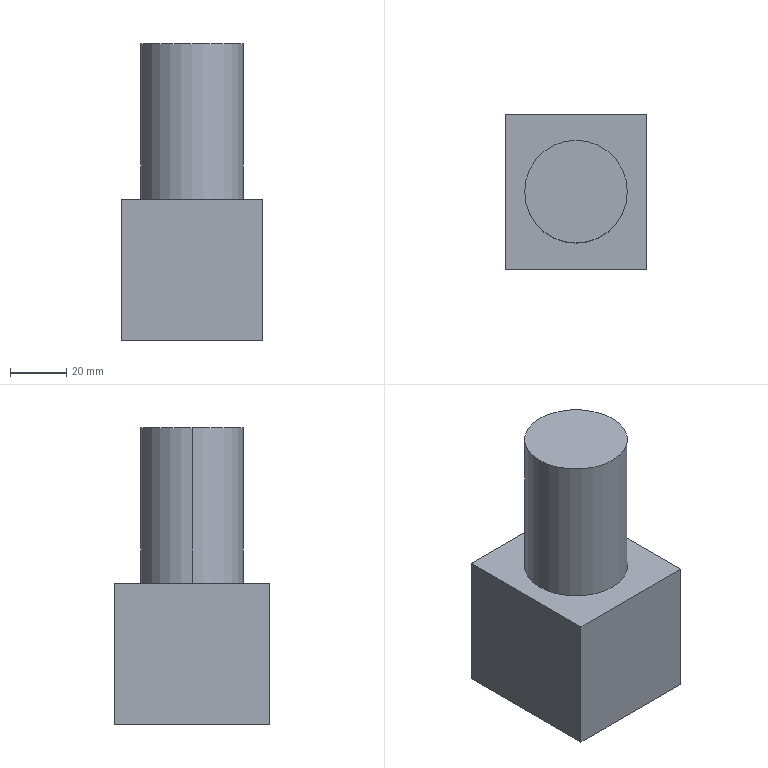Part | SolidWorks | features Extrusion 1, ICE 1 | 1 solid | 9 faces | box 50 x 55 x 105 mm | volume 194665 mm3 | plane 7 | cylinder 2 | commonest cylinder face diameters 36.378 x2
STEP:
#1=CARTESIAN_POINT('',(18.189,27.5,80.));
#2=VERTEX_POINT('',#1);
#3=CARTESIAN_POINT('',(-18.189,27.5,80.));
#4=VERTEX_POINT('',#3);
#5=CARTESIAN_POINT('',(0.,27.5,80.));
#6=DIRECTION('',(0.,0.,1.));
#7=DIRECTION('',(1.,0.,0.));
#8=AXIS2_PLACEMENT_3D('',#5,#6,#7);
#9=CIRCLE('',#8,18.189);
#10=EDGE_CURVE('',#2,#4,#9,.T.);
#11=ORIENTED_EDGE('',*,*,#10,.F.);
#12=CARTESIAN_POINT('',(18.189,27.5,25.));
#13=VERTEX_POINT('',#12);
#14=CARTESIAN_POINT('',(18.189,27.5,80.));
#15=DIRECTION('',(0.,0.,-1.));
#16=VECTOR('',#15,1000.);
#17=LINE('',#14,#16);
#18=EDGE_CURVE('',#2,#13,#17,.T.);
#19=ORIENTED_EDGE('',*,*,#18,.T.);
#20=CARTESIAN_POINT('',(-18.189,27.5,25.));
#21=VERTEX_POINT('',#20);
#22=CARTESIAN_POINT('',(0.,27.5,25.));
#23=DIRECTION('',(0.,0.,1.));
#24=DIRECTION('',(1.,0.,0.));
#25=AXIS2_PLACEMENT_3D('',#22,#23,#24);
#26=CIRCLE('',#25,18.189);
#27=EDGE_CURVE('',#13,#21,#26,.T.);
#28=ORIENTED_EDGE('',*,*,#27,.T.);
#29=CARTESIAN_POINT('',(-18.189,27.5,80.));
#30=DIRECTION('',(0.,0.,-1.));
#31=VECTOR('',#30,1000.);
#32=LINE('',#29,#31);
#33=EDGE_CURVE('',#4,#21,#32,.T.);
#34=ORIENTED_EDGE('',*,*,#33,.F.);
#35=EDGE_LOOP('',(#11,#19,#28,#34));
#36=FACE_OUTER_BOUND('',#35,.T.);
#37=CARTESIAN_POINT('',(0.,27.5,80.));
#38=DIRECTION('',(0.,0.,-1.));
#39=DIRECTION('',(-1.,0.,0.));
#40=AXIS2_PLACEMENT_3D('',#37,#38,#39);
#41=CYLINDRICAL_SURFACE('',#40,18.189);
#42=ADVANCED_FACE('',(#36),#41,.T.);
#43=CARTESIAN_POINT('',(25.,0.,25.));
#44=VERTEX_POINT('',#43);
#45=CARTESIAN_POINT('',(25.,0.,-25.));
#46=VERTEX_POINT('',#45);
#47=CARTESIAN_POINT('',(25.,0.,-25.));
#48=DIRECTION('',(0.,0.,-1.));
#49=VECTOR('',#48,1000.);
#50=LINE('',#47,#49);
#51=EDGE_CURVE('',#44,#46,#50,.T.);
#52=ORIENTED_EDGE('',*,*,#51,.T.);
#53=CARTESIAN_POINT('',(25.,55.,-25.));
#54=VERTEX_POINT('',#53);
#55=CARTESIAN_POINT('',(25.,55.,-25.));
#56=DIRECTION('',(0.,-1.,0.));
#57=VECTOR('',#56,1000.);
#58=LINE('',#55,#57);
#59=EDGE_CURVE('',#54,#46,#58,.T.);
#60=ORIENTED_EDGE('',*,*,#59,.F.);
#61=CARTESIAN_POINT('',(25.,55.,25.));
#62=VERTEX_POINT('',#61);
#63=CARTESIAN_POINT('',(25.,55.,-25.));
#64=DIRECTION('',(0.,0.,-1.));
#65=VECTOR('',#64,1000.);
#66=LINE('',#63,#65);
#67=EDGE_CURVE('',#62,#54,#66,.T.);
#68=ORIENTED_EDGE('',*,*,#67,.F.);
#69=CARTESIAN_POINT('',(25.,55.,25.));
#70=DIRECTION('',(0.,-1.,0.));
#71=VECTOR('',#70,1000.);
#72=LINE('',#69,#71);
#73=EDGE_CURVE('',#62,#44,#72,.T.);
#74=ORIENTED_EDGE('',*,*,#73,.T.);
#75=EDGE_LOOP('',(#52,#60,#68,#74));
#76=FACE_OUTER_BOUND('',#75,.T.);
#77=CARTESIAN_POINT('',(25.,55.,-25.));
#78=DIRECTION('',(-1.,0.,0.));
#79=DIRECTION('',(0.,0.,1.));
#80=AXIS2_PLACEMENT_3D('',#77,#78,#79);
#81=PLANE('',#80);
#82=ADVANCED_FACE('',(#76),#81,.F.);
#83=CARTESIAN_POINT('',(-25.,0.,-25.));
#84=VERTEX_POINT('',#83);
#85=CARTESIAN_POINT('',(-25.,0.,-25.));
#86=DIRECTION('',(-1.,0.,0.));
#87=VECTOR('',#86,1000.);
#88=LINE('',#85,#87);
#89=EDGE_CURVE('',#46,#84,#88,.T.);
#90=ORIENTED_EDGE('',*,*,#89,.T.);
#91=CARTESIAN_POINT('',(-25.,55.,-25.));
#92=VERTEX_POINT('',#91);
#93=CARTESIAN_POINT('',(-25.,55.,-25.));
#94=DIRECTION('',(0.,-1.,0.));
#95=VECTOR('',#94,1000.);
#96=LINE('',#93,#95);
#97=EDGE_CURVE('',#92,#84,#96,.T.);
#98=ORIENTED_EDGE('',*,*,#97,.F.);
#99=CARTESIAN_POINT('',(-25.,55.,-25.));
#100=DIRECTION('',(-1.,0.,0.));
#101=VECTOR('',#100,1000.);
#102=LINE('',#99,#101);
#103=EDGE_CURVE('',#54,#92,#102,.T.);
#104=ORIENTED_EDGE('',*,*,#103,.F.);
#105=ORIENTED_EDGE('',*,*,#59,.T.);
#106=EDGE_LOOP('',(#90,#98,#104,#105));
#107=FACE_OUTER_BOUND('',#106,.T.);
#108=CARTESIAN_POINT('',(-25.,55.,-25.));
#109=DIRECTION('',(0.,0.,1.));
#110=DIRECTION('',(1.,0.,0.));
#111=AXIS2_PLACEMENT_3D('',#108,#109,#110);
#112=PLANE('',#111);
#113=ADVANCED_FACE('',(#107),#112,.F.);
#114=CARTESIAN_POINT('',(-25.,0.,25.));
#115=VERTEX_POINT('',#114);
#116=CARTESIAN_POINT('',(-25.,0.,-25.));
#117=DIRECTION('',(0.,0.,1.));
#118=VECTOR('',#117,1000.);
#119=LINE('',#116,#118);
#120=EDGE_CURVE('',#84,#115,#119,.T.);
#121=ORIENTED_EDGE('',*,*,#120,.T.);
#122=CARTESIAN_POINT('',(-25.,55.,25.));
#123=VERTEX_POINT('',#122);
#124=CARTESIAN_POINT('',(-25.,55.,25.));
#125=DIRECTION('',(0.,-1.,0.));
#126=VECTOR('',#125,1000.);
#127=LINE('',#124,#126);
#128=EDGE_CURVE('',#123,#115,#127,.T.);
#129=ORIENTED_EDGE('',*,*,#128,.F.);
#130=CARTESIAN_POINT('',(-25.,55.,-25.));
#131=DIRECTION('',(0.,0.,1.));
#132=VECTOR('',#131,1000.);
#133=LINE('',#130,#132);
#134=EDGE_CURVE('',#92,#123,#133,.T.);
#135=ORIENTED_EDGE('',*,*,#134,.F.);
#136=ORIENTED_EDGE('',*,*,#97,.T.);
#137=EDGE_LOOP('',(#121,#129,#135,#136));
#138=FACE_OUTER_BOUND('',#137,.T.);
#139=CARTESIAN_POINT('',(-25.,55.,-25.));
#140=DIRECTION('',(1.,0.,0.));
#141=DIRECTION('',(0.,0.,-1.));
#142=AXIS2_PLACEMENT_3D('',#139,#140,#141);
#143=PLANE('',#142);
#144=ADVANCED_FACE('',(#138),#143,.F.);
#145=CARTESIAN_POINT('',(0.,27.5,25.));
#146=DIRECTION('',(0.,0.,1.));
#147=DIRECTION('',(1.,0.,0.));
#148=AXIS2_PLACEMENT_3D('',#145,#146,#147);
#149=CIRCLE('',#148,18.189);
#150=EDGE_CURVE('',#21,#13,#149,.T.);
#151=ORIENTED_EDGE('',*,*,#150,.F.);
#152=ORIENTED_EDGE('',*,*,#27,.F.);
#153=EDGE_LOOP('',(#151,#152));
#154=FACE_BOUND('',#153,.T.);
#155=CARTESIAN_POINT('',(-25.,0.,25.));
#156=DIRECTION('',(1.,0.,0.));
#157=VECTOR('',#156,1000.);
#158=LINE('',#155,#157);
#159=EDGE_CURVE('',#115,#44,#158,.T.);
#160=ORIENTED_EDGE('',*,*,#159,.T.);
#161=ORIENTED_EDGE('',*,*,#73,.F.);
#162=CARTESIAN_POINT('',(-25.,55.,25.));
#163=DIRECTION('',(1.,0.,0.));
#164=VECTOR('',#163,1000.);
#165=LINE('',#162,#164);
#166=EDGE_CURVE('',#123,#62,#165,.T.);
#167=ORIENTED_EDGE('',*,*,#166,.F.);
#168=ORIENTED_EDGE('',*,*,#128,.T.);
#169=EDGE_LOOP('',(#160,#161,#167,#168));
#170=FACE_OUTER_BOUND('',#169,.T.);
#171=CARTESIAN_POINT('',(-25.,55.,25.));
#172=DIRECTION('',(0.,0.,-1.));
#173=DIRECTION('',(-1.,0.,0.));
#174=AXIS2_PLACEMENT_3D('',#171,#172,#173);
#175=PLANE('',#174);
#176=ADVANCED_FACE('',(#154,#170),#175,.F.);
#177=ORIENTED_EDGE('',*,*,#67,.T.);
#178=ORIENTED_EDGE('',*,*,#103,.T.);
#179=ORIENTED_EDGE('',*,*,#134,.T.);
#180=ORIENTED_EDGE('',*,*,#166,.T.);
#181=EDGE_LOOP('',(#177,#178,#179,#180));
#182=FACE_OUTER_BOUND('',#181,.T.);
#183=CARTESIAN_POINT('',(0.,55.,0.));
#184=DIRECTION('',(0.,1.,0.));
#185=DIRECTION('',(0.,0.,1.));
#186=AXIS2_PLACEMENT_3D('',#183,#184,#185);
#187=PLANE('',#186);
#188=ADVANCED_FACE('',(#182),#187,.T.);
#189=ORIENTED_EDGE('',*,*,#51,.F.);
#190=ORIENTED_EDGE('',*,*,#159,.F.);
#191=ORIENTED_EDGE('',*,*,#120,.F.);
#192=ORIENTED_EDGE('',*,*,#89,.F.);
#193=EDGE_LOOP('',(#189,#190,#191,#192));
#194=FACE_OUTER_BOUND('',#193,.T.);
#195=CARTESIAN_POINT('',(0.,0.,0.));
#196=DIRECTION('',(0.,1.,0.));
#197=DIRECTION('',(0.,0.,1.));
#198=AXIS2_PLACEMENT_3D('',#195,#196,#197);
#199=PLANE('',#198);
#200=ADVANCED_FACE('',(#194),#199,.F.);
#201=ORIENTED_EDGE('',*,*,#18,.F.);
#202=CARTESIAN_POINT('',(0.,27.5,80.));
#203=DIRECTION('',(0.,0.,1.));
#204=DIRECTION('',(1.,0.,0.));
#205=AXIS2_PLACEMENT_3D('',#202,#203,#204);
#206=CIRCLE('',#205,18.189);
#207=EDGE_CURVE('',#4,#2,#206,.T.);
#208=ORIENTED_EDGE('',*,*,#207,.F.);
#209=ORIENTED_EDGE('',*,*,#33,.T.);
#210=ORIENTED_EDGE('',*,*,#150,.T.);
#211=EDGE_LOOP('',(#201,#208,#209,#210));
#212=FACE_OUTER_BOUND('',#211,.T.);
#213=CARTESIAN_POINT('',(0.,27.5,80.));
#214=DIRECTION('',(0.,0.,-1.));
#215=DIRECTION('',(-1.,0.,0.));
#216=AXIS2_PLACEMENT_3D('',#213,#214,#215);
#217=CYLINDRICAL_SURFACE('',#216,18.189);
#218=ADVANCED_FACE('',(#212),#217,.T.);
#219=ORIENTED_EDGE('',*,*,#207,.T.);
#220=ORIENTED_EDGE('',*,*,#10,.T.);
#221=EDGE_LOOP('',(#219,#220));
#222=FACE_OUTER_BOUND('',#221,.T.);
#223=CARTESIAN_POINT('',(0.,27.5,80.));
#224=DIRECTION('',(0.,0.,1.));
#225=DIRECTION('',(1.,0.,0.));
#226=AXIS2_PLACEMENT_3D('',#223,#224,#225);
#227=PLANE('',#226);
#228=ADVANCED_FACE('',(#222),#227,.T.);
#229=CLOSED_SHELL('',(#42,#82,#113,#144,#176,#188,#200,#218,#228));
#230=MANIFOLD_SOLID_BREP('',#229);
#231=CARTESIAN_POINT('',(0.,0.,0.));
#232=DIRECTION('',(0.,0.,1.));
#233=DIRECTION('',(1.,0.,0.));
#234=AXIS2_PLACEMENT_3D('',#231,#232,#233);
#235=(LENGTH_UNIT()NAMED_UNIT(*)SI_UNIT(.MILLI.,.METRE.));
#236=UNCERTAINTY_MEASURE_WITH_UNIT(LENGTH_MEASURE(0.00001),#235,'','');
#237=(NAMED_UNIT(*)PLANE_ANGLE_UNIT()SI_UNIT($,.RADIAN.));
#238=(NAMED_UNIT(*)SI_UNIT($,.STERADIAN.)SOLID_ANGLE_UNIT());
#239=(GEOMETRIC_REPRESENTATION_CONTEXT(3)GLOBAL_UNCERTAINTY_ASSIGNED_CONTEXT((#236))GLOBAL_UNIT_ASSIGNED_CONTEXT((#235,#237,#238))REPRESENTATION_CONTEXT('',''));
#240=ADVANCED_BREP_SHAPE_REPRESENTATION('',(#230,#234),#239);